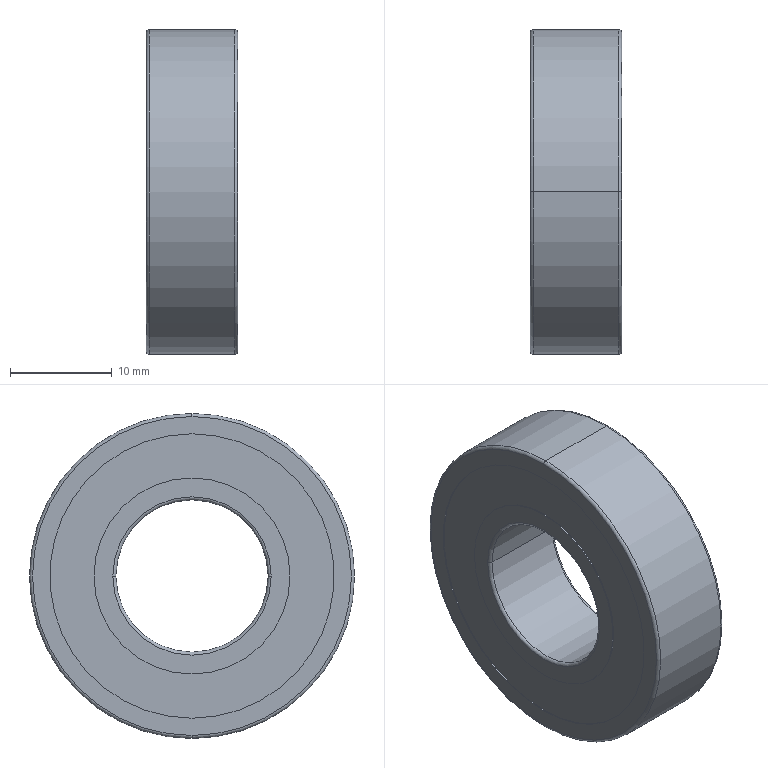Part | SolidWorks | features BaseBody 17 | 17 solids | 80 faces | box 9 x 32 x 32 mm | volume 4096 mm3 | cylinder 28 | sphere 26 | torus 14 | plane 12 | commonest cylinder face diameters 19.3 x8 28 x8 20.5 x4 26.5 x4 15 x2 32 x2